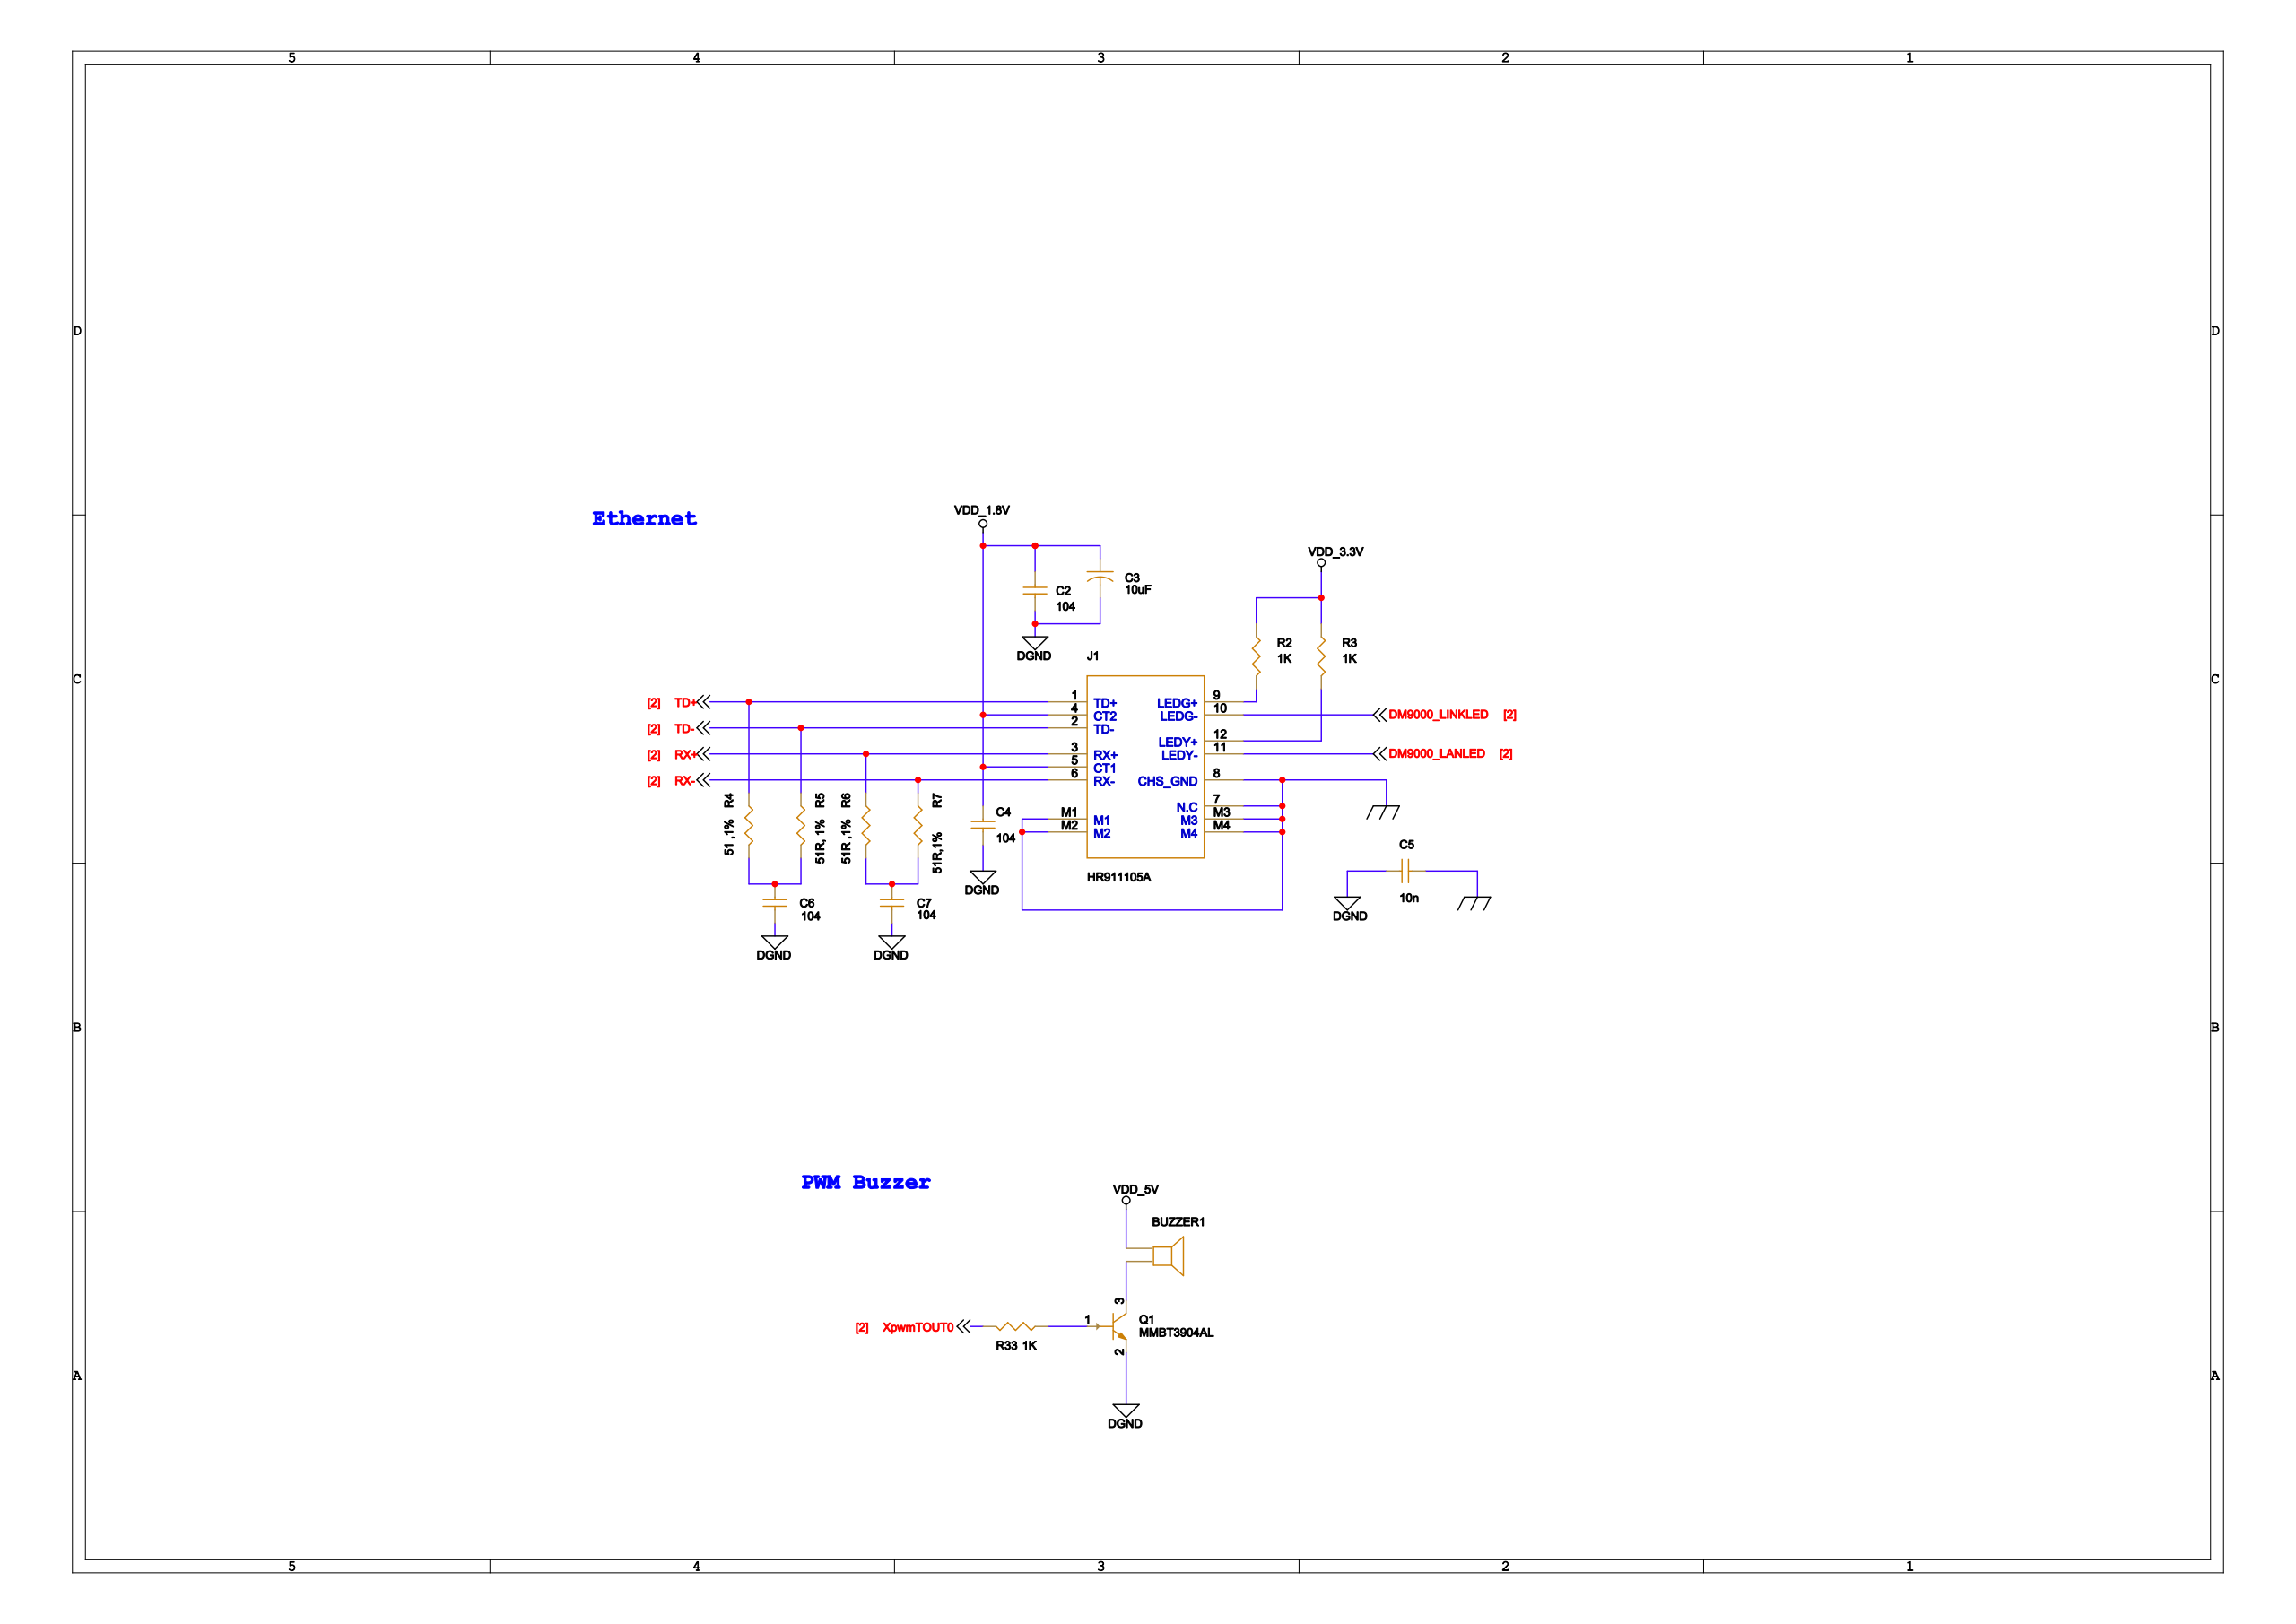Circuit board | Cadence Allegro | 85 parts | 48 nets | one sheet of the schematic
Parts on this sheet (reference | value | footprint):
BUZZER1 | SPEAKER | FM1
C2 | 104 | C0603
C3 | 10uF | C0805
C4 | 104 | C0603
C5 | 10n | C0603
C6 | 104 | C0603
C7 | 104 | C0603
J1 | HR911105A | HR911105A
Q1 | MMBT3904AL | SOT-23-D
R3 | 1K | R0603
R4 | 51 ,1% | R0603
R5 | 51R, 1% | R0603
R6 | 51R ,1% | R0603
R7 | 51R,1% | R0603
R33 | 1K | R0603
Nets of these parts (net: part-pin ...):
VDD_5V: BUZZER1-1
DGND: C2-2 C3-2 C4-2 C5-1 C6-2 C7-2 Q1-2
N9826499: Q1-1 R33-1
N9833466: BUZZER1-2 Q1-3
VDD_1.8V: C2-1 C3-1 C4-1 J1-4 J1-5
GND_EARTH: C5-2 J1-7 J1-8 J1-M1 J1-M2 J1-M3 J1-M4
N9800656: J1-9
DM9000_LINKLED: J1-10
N9800680: J1-12 R3-2
DM9000_LANLED: J1-11
RX+: J1-3 R6-1
RX-: J1-6 R7-1
TD+: J1-1 R4-1
TD-: J1-2 R5-1
VDD_3.3V: R3-1
N9800628: C6-1 R4-2 R5-2
N9800688: C7-1 R6-2 R7-2
XPWMTOUT0: R33-2